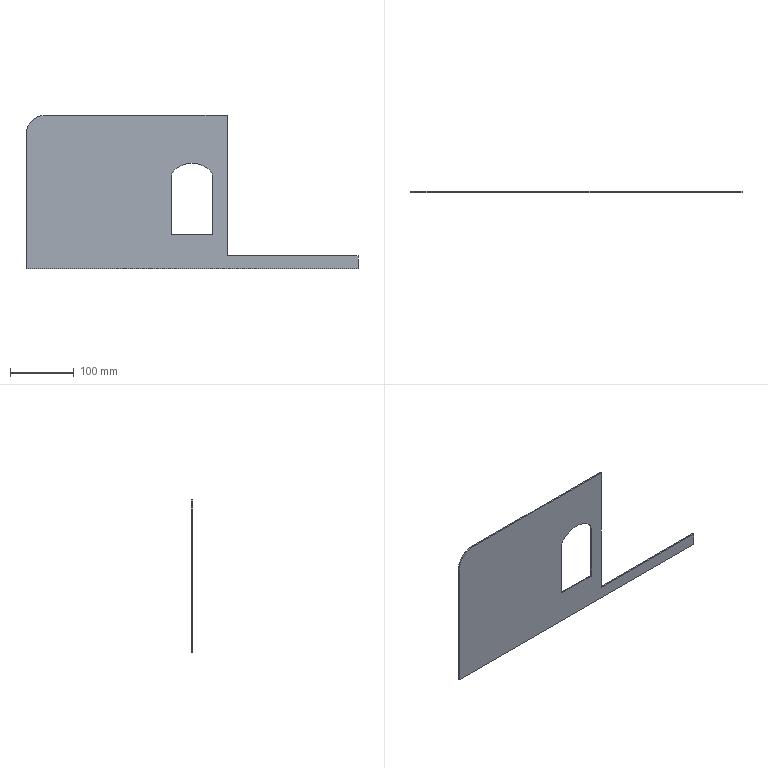Part | STEP file | A14-052 | 1 solid | 16 faces | box 520 x 2 x 240 mm | volume 145187 mm3 | plane 11 | cylinder 5 | commonest cylinder face diameters 25.5 x2 79.6 x2 60 x1
STEP:
#1=CARTESIAN_POINT('',(0.,0.,0.));
#2=DIRECTION('',(0.,0.,1.));
#3=DIRECTION('',(1.,0.,0.));
#4=AXIS2_PLACEMENT_3D('',#1,#2,#3);
#5=CARTESIAN_POINT('',(28.765,-1.,32.757));
#6=VERTEX_POINT('',#5);
#7=CARTESIAN_POINT('',(28.765,1.,32.757));
#8=VERTEX_POINT('',#7);
#9=CARTESIAN_POINT('',(28.765,-9.,32.757));
#10=DIRECTION('',(0.,1.,0.));
#11=VECTOR('',#10,1.);
#12=LINE('',#9,#11);
#13=CARTESIAN_POINT('',(0.,-9.,5.25));
#14=DIRECTION('',(0.,1.,0.));
#15=DIRECTION('',(0.,0.,1.));
#16=AXIS2_PLACEMENT_3D('',#13,#14,#15);
#17=CYLINDRICAL_SURFACE('',#16,39.8);
#18=CARTESIAN_POINT('',(0.8078,0.));
#19=DIRECTION('',(0.,1.));
#20=VECTOR('',#19,1.);
#21=LINE('',#18,#20);
#22=(GEOMETRIC_REPRESENTATION_CONTEXT(2)PARAMETRIC_REPRESENTATION_CONTEXT()REPRESENTATION_CONTEXT('',''));
#23=DEFINITIONAL_REPRESENTATION('',(#21),#22);
#24=PCURVE('',#17,#23);
#25=CARTESIAN_POINT('',(19.55,-9.,23.945));
#26=DIRECTION('',(0.,1.,0.));
#27=DIRECTION('',(0.,0.,1.));
#28=AXIS2_PLACEMENT_3D('',#25,#26,#27);
#29=CYLINDRICAL_SURFACE('',#28,12.75);
#30=CARTESIAN_POINT('',(0.8078,0.));
#31=DIRECTION('',(0.,1.));
#32=VECTOR('',#31,1.);
#33=LINE('',#30,#32);
#34=(GEOMETRIC_REPRESENTATION_CONTEXT(2)PARAMETRIC_REPRESENTATION_CONTEXT()REPRESENTATION_CONTEXT('',''));
#35=DEFINITIONAL_REPRESENTATION('',(#33),#34);
#36=PCURVE('',#29,#35);
#37=SURFACE_CURVE('',#12,(#24,#36),.PCURVE_S1.);
#38=EDGE_CURVE('',#6,#8,#37,.T.);
#39=ORIENTED_EDGE('',*,*,#38,.T.);
#40=CARTESIAN_POINT('',(0.,1.,45.05));
#41=VERTEX_POINT('',#40);
#42=CARTESIAN_POINT('',(0.,1.,5.25));
#43=DIRECTION('',(0.,1.,0.));
#44=DIRECTION('',(0.,0.,1.));
#45=AXIS2_PLACEMENT_3D('',#42,#43,#44);
#46=CIRCLE('',#45,39.8);
#47=CARTESIAN_POINT('',(0.,10.));
#48=DIRECTION('',(1.,0.));
#49=VECTOR('',#48,1.);
#50=LINE('',#47,#49);
#51=(GEOMETRIC_REPRESENTATION_CONTEXT(2)PARAMETRIC_REPRESENTATION_CONTEXT()REPRESENTATION_CONTEXT('',''));
#52=DEFINITIONAL_REPRESENTATION('',(#50),#51);
#53=PCURVE('',#17,#52);
#54=CARTESIAN_POINT('',(0.,1.,0.));
#55=DIRECTION('',(0.,1.,0.));
#56=DIRECTION('',(0.,0.,1.));
#57=AXIS2_PLACEMENT_3D('',#54,#55,#56);
#58=PLANE('',#57);
#59=CARTESIAN_POINT('',(5.25,0.));
#60=DIRECTION('',(1.,0.));
#61=AXIS2_PLACEMENT_2D('',#59,#60);
#62=CIRCLE('',#61,39.8);
#63=(GEOMETRIC_REPRESENTATION_CONTEXT(2)PARAMETRIC_REPRESENTATION_CONTEXT()REPRESENTATION_CONTEXT('',''));
#64=DEFINITIONAL_REPRESENTATION('',(#62),#63);
#65=PCURVE('',#58,#64);
#66=SURFACE_CURVE('',#46,(#53,#65),.PCURVE_S1.);
#67=EDGE_CURVE('',#41,#8,#66,.T.);
#68=ORIENTED_EDGE('',*,*,#67,.F.);
#69=CARTESIAN_POINT('',(0.,-1.,45.05));
#70=VERTEX_POINT('',#69);
#71=CARTESIAN_POINT('',(0.,-9.,45.05));
#72=DIRECTION('',(0.,1.,0.));
#73=VECTOR('',#72,1.);
#74=LINE('',#71,#73);
#75=CARTESIAN_POINT('',(0.,0.));
#76=DIRECTION('',(0.,1.));
#77=VECTOR('',#76,1.);
#78=LINE('',#75,#77);
#79=(GEOMETRIC_REPRESENTATION_CONTEXT(2)PARAMETRIC_REPRESENTATION_CONTEXT()REPRESENTATION_CONTEXT('',''));
#80=DEFINITIONAL_REPRESENTATION('',(#78),#79);
#81=PCURVE('',#17,#80);
#82=CARTESIAN_POINT('',(0.,-9.,5.25));
#83=DIRECTION('',(0.,1.,0.));
#84=DIRECTION('',(0.,0.,1.));
#85=AXIS2_PLACEMENT_3D('',#82,#83,#84);
#86=CYLINDRICAL_SURFACE('',#85,39.8);
#87=CARTESIAN_POINT('',(6.283,0.));
#88=DIRECTION('',(0.,1.));
#89=VECTOR('',#88,1.);
#90=LINE('',#87,#89);
#91=(GEOMETRIC_REPRESENTATION_CONTEXT(2)PARAMETRIC_REPRESENTATION_CONTEXT()REPRESENTATION_CONTEXT('',''));
#92=DEFINITIONAL_REPRESENTATION('',(#90),#91);
#93=PCURVE('',#86,#92);
#94=SURFACE_CURVE('',#74,(#81,#93),.PCURVE_S1.);
#95=EDGE_CURVE('',#70,#41,#94,.T.);
#96=ORIENTED_EDGE('',*,*,#95,.F.);
#97=CARTESIAN_POINT('',(0.,-1.,5.25));
#98=DIRECTION('',(0.,1.,0.));
#99=DIRECTION('',(0.,0.,1.));
#100=AXIS2_PLACEMENT_3D('',#97,#98,#99);
#101=CIRCLE('',#100,39.8);
#102=CARTESIAN_POINT('',(0.,8.));
#103=DIRECTION('',(1.,0.));
#104=VECTOR('',#103,1.);
#105=LINE('',#102,#104);
#106=(GEOMETRIC_REPRESENTATION_CONTEXT(2)PARAMETRIC_REPRESENTATION_CONTEXT()REPRESENTATION_CONTEXT('',''));
#107=DEFINITIONAL_REPRESENTATION('',(#105),#106);
#108=PCURVE('',#17,#107);
#109=CARTESIAN_POINT('',(0.,-1.,0.));
#110=DIRECTION('',(0.,1.,0.));
#111=DIRECTION('',(0.,0.,1.));
#112=AXIS2_PLACEMENT_3D('',#109,#110,#111);
#113=PLANE('',#112);
#114=CARTESIAN_POINT('',(5.25,0.));
#115=DIRECTION('',(1.,0.));
#116=AXIS2_PLACEMENT_2D('',#114,#115);
#117=CIRCLE('',#116,39.8);
#118=(GEOMETRIC_REPRESENTATION_CONTEXT(2)PARAMETRIC_REPRESENTATION_CONTEXT()REPRESENTATION_CONTEXT('',''));
#119=DEFINITIONAL_REPRESENTATION('',(#117),#118);
#120=PCURVE('',#113,#119);
#121=SURFACE_CURVE('',#101,(#108,#120),.PCURVE_S1.);
#122=EDGE_CURVE('',#70,#6,#121,.T.);
#123=ORIENTED_EDGE('',*,*,#122,.T.);
#124=EDGE_LOOP('',(#39,#68,#96,#123));
#125=FACE_BOUND('',#124,.F.);
#126=ADVANCED_FACE('',(#125),#17,.F.);
#127=CARTESIAN_POINT('',(260.,1.,-100.));
#128=VERTEX_POINT('',#127);
#129=CARTESIAN_POINT('',(260.,1.,-120.));
#130=VERTEX_POINT('',#129);
#131=CARTESIAN_POINT('',(260.,1.,-120.));
#132=DIRECTION('',(0.,0.,-1.));
#133=VECTOR('',#132,1.);
#134=LINE('',#131,#133);
#135=CARTESIAN_POINT('',(260.,1.,-120.));
#136=DIRECTION('',(-1.,0.,0.));
#137=DIRECTION('',(0.,0.,1.));
#138=AXIS2_PLACEMENT_3D('',#135,#136,#137);
#139=PLANE('',#138);
#140=CARTESIAN_POINT('',(0.,0.));
#141=DIRECTION('',(-1.,0.));
#142=VECTOR('',#141,1.);
#143=LINE('',#140,#142);
#144=(GEOMETRIC_REPRESENTATION_CONTEXT(2)PARAMETRIC_REPRESENTATION_CONTEXT()REPRESENTATION_CONTEXT('',''));
#145=DEFINITIONAL_REPRESENTATION('',(#143),#144);
#146=PCURVE('',#139,#145);
#147=CARTESIAN_POINT('',(-120.,260.));
#148=DIRECTION('',(-1.,0.));
#149=VECTOR('',#148,1.);
#150=LINE('',#147,#149);
#151=(GEOMETRIC_REPRESENTATION_CONTEXT(2)PARAMETRIC_REPRESENTATION_CONTEXT()REPRESENTATION_CONTEXT('',''));
#152=DEFINITIONAL_REPRESENTATION('',(#150),#151);
#153=PCURVE('',#58,#152);
#154=SURFACE_CURVE('',#134,(#146,#153),.PCURVE_S1.);
#155=EDGE_CURVE('',#128,#130,#154,.T.);
#156=ORIENTED_EDGE('',*,*,#155,.F.);
#157=CARTESIAN_POINT('',(260.,-1.,-100.));
#158=VERTEX_POINT('',#157);
#159=CARTESIAN_POINT('',(260.,-9.,-100.));
#160=DIRECTION('',(0.,1.,0.));
#161=VECTOR('',#160,1.);
#162=LINE('',#159,#161);
#163=CARTESIAN_POINT('',(20.,-10.));
#164=DIRECTION('',(0.,1.));
#165=VECTOR('',#164,1.);
#166=LINE('',#163,#165);
#167=(GEOMETRIC_REPRESENTATION_CONTEXT(2)PARAMETRIC_REPRESENTATION_CONTEXT()REPRESENTATION_CONTEXT('',''));
#168=DEFINITIONAL_REPRESENTATION('',(#166),#167);
#169=PCURVE('',#139,#168);
#170=CARTESIAN_POINT('',(55.,-9.,-100.));
#171=DIRECTION('',(0.,0.,-1.));
#172=DIRECTION('',(-1.,0.,0.));
#173=AXIS2_PLACEMENT_3D('',#170,#171,#172);
#174=PLANE('',#173);
#175=CARTESIAN_POINT('',(-205.,0.));
#176=DIRECTION('',(0.,1.));
#177=VECTOR('',#176,1.);
#178=LINE('',#175,#177);
#179=(GEOMETRIC_REPRESENTATION_CONTEXT(2)PARAMETRIC_REPRESENTATION_CONTEXT()REPRESENTATION_CONTEXT('',''));
#180=DEFINITIONAL_REPRESENTATION('',(#178),#179);
#181=PCURVE('',#174,#180);
#182=SURFACE_CURVE('',#162,(#169,#181),.PCURVE_S1.);
#183=EDGE_CURVE('',#158,#128,#182,.T.);
#184=ORIENTED_EDGE('',*,*,#183,.F.);
#185=CARTESIAN_POINT('',(260.,-1.,-120.));
#186=VERTEX_POINT('',#185);
#187=CARTESIAN_POINT('',(260.,-1.,-120.));
#188=DIRECTION('',(0.,0.,-1.));
#189=VECTOR('',#188,1.);
#190=LINE('',#187,#189);
#191=CARTESIAN_POINT('',(0.,-2.));
#192=DIRECTION('',(-1.,0.));
#193=VECTOR('',#192,1.);
#194=LINE('',#191,#193);
#195=(GEOMETRIC_REPRESENTATION_CONTEXT(2)PARAMETRIC_REPRESENTATION_CONTEXT()REPRESENTATION_CONTEXT('',''));
#196=DEFINITIONAL_REPRESENTATION('',(#194),#195);
#197=PCURVE('',#139,#196);
#198=CARTESIAN_POINT('',(-120.,260.));
#199=DIRECTION('',(-1.,0.));
#200=VECTOR('',#199,1.);
#201=LINE('',#198,#200);
#202=(GEOMETRIC_REPRESENTATION_CONTEXT(2)PARAMETRIC_REPRESENTATION_CONTEXT()REPRESENTATION_CONTEXT('',''));
#203=DEFINITIONAL_REPRESENTATION('',(#201),#202);
#204=PCURVE('',#113,#203);
#205=SURFACE_CURVE('',#190,(#197,#204),.PCURVE_S1.);
#206=EDGE_CURVE('',#158,#186,#205,.T.);
#207=ORIENTED_EDGE('',*,*,#206,.T.);
#208=CARTESIAN_POINT('',(260.,1.,-120.));
#209=DIRECTION('',(0.,-1.,0.));
#210=VECTOR('',#209,1.);
#211=LINE('',#208,#210);
#212=CARTESIAN_POINT('',(0.,0.));
#213=DIRECTION('',(0.,-1.));
#214=VECTOR('',#213,1.);
#215=LINE('',#212,#214);
#216=(GEOMETRIC_REPRESENTATION_CONTEXT(2)PARAMETRIC_REPRESENTATION_CONTEXT()REPRESENTATION_CONTEXT('',''));
#217=DEFINITIONAL_REPRESENTATION('',(#215),#216);
#218=PCURVE('',#139,#217);
#219=CARTESIAN_POINT('',(-260.,1.,-120.));
#220=DIRECTION('',(0.,0.,1.));
#221=DIRECTION('',(1.,0.,0.));
#222=AXIS2_PLACEMENT_3D('',#219,#220,#221);
#223=PLANE('',#222);
#224=CARTESIAN_POINT('',(520.,0.));
#225=DIRECTION('',(0.,-1.));
#226=VECTOR('',#225,1.);
#227=LINE('',#224,#226);
#228=(GEOMETRIC_REPRESENTATION_CONTEXT(2)PARAMETRIC_REPRESENTATION_CONTEXT()REPRESENTATION_CONTEXT('',''));
#229=DEFINITIONAL_REPRESENTATION('',(#227),#228);
#230=PCURVE('',#223,#229);
#231=SURFACE_CURVE('',#211,(#218,#230),.PCURVE_S1.);
#232=EDGE_CURVE('',#130,#186,#231,.T.);
#233=ORIENTED_EDGE('',*,*,#232,.F.);
#234=EDGE_LOOP('',(#156,#184,#207,#233));
#235=FACE_BOUND('',#234,.T.);
#236=ADVANCED_FACE('',(#235),#139,.F.);
#237=CARTESIAN_POINT('',(-260.,-1.,-120.));
#238=VERTEX_POINT('',#237);
#239=CARTESIAN_POINT('',(-260.,-1.,-120.));
#240=DIRECTION('',(-1.,0.,0.));
#241=VECTOR('',#240,1.);
#242=LINE('',#239,#241);
#243=CARTESIAN_POINT('',(0.,-2.));
#244=DIRECTION('',(-1.,0.));
#245=VECTOR('',#244,1.);
#246=LINE('',#243,#245);
#247=(GEOMETRIC_REPRESENTATION_CONTEXT(2)PARAMETRIC_REPRESENTATION_CONTEXT()REPRESENTATION_CONTEXT('',''));
#248=DEFINITIONAL_REPRESENTATION('',(#246),#247);
#249=PCURVE('',#223,#248);
#250=CARTESIAN_POINT('',(-120.,-260.));
#251=DIRECTION('',(0.,-1.));
#252=VECTOR('',#251,1.);
#253=LINE('',#250,#252);
#254=(GEOMETRIC_REPRESENTATION_CONTEXT(2)PARAMETRIC_REPRESENTATION_CONTEXT()REPRESENTATION_CONTEXT('',''));
#255=DEFINITIONAL_REPRESENTATION('',(#253),#254);
#256=PCURVE('',#113,#255);
#257=SURFACE_CURVE('',#242,(#249,#256),.PCURVE_S1.);
#258=EDGE_CURVE('',#186,#238,#257,.T.);
#259=ORIENTED_EDGE('',*,*,#258,.T.);
#260=CARTESIAN_POINT('',(-260.,1.,-120.));
#261=VERTEX_POINT('',#260);
#262=CARTESIAN_POINT('',(-260.,1.,-120.));
#263=DIRECTION('',(0.,-1.,0.));
#264=VECTOR('',#263,1.);
#265=LINE('',#262,#264);
#266=CARTESIAN_POINT('',(0.,0.));
#267=DIRECTION('',(0.,-1.));
#268=VECTOR('',#267,1.);
#269=LINE('',#266,#268);
#270=(GEOMETRIC_REPRESENTATION_CONTEXT(2)PARAMETRIC_REPRESENTATION_CONTEXT()REPRESENTATION_CONTEXT('',''));
#271=DEFINITIONAL_REPRESENTATION('',(#269),#270);
#272=PCURVE('',#223,#271);
#273=CARTESIAN_POINT('',(-260.,1.,-120.));
#274=DIRECTION('',(1.,0.,0.));
#275=DIRECTION('',(0.,0.,-1.));
#276=AXIS2_PLACEMENT_3D('',#273,#274,#275);
#277=PLANE('',#276);
#278=CARTESIAN_POINT('',(0.,0.));
#279=DIRECTION('',(0.,-1.));
#280=VECTOR('',#279,1.);
#281=LINE('',#278,#280);
#282=(GEOMETRIC_REPRESENTATION_CONTEXT(2)PARAMETRIC_REPRESENTATION_CONTEXT()REPRESENTATION_CONTEXT('',''));
#283=DEFINITIONAL_REPRESENTATION('',(#281),#282);
#284=PCURVE('',#277,#283);
#285=SURFACE_CURVE('',#265,(#272,#284),.PCURVE_S1.);
#286=EDGE_CURVE('',#261,#238,#285,.T.);
#287=ORIENTED_EDGE('',*,*,#286,.F.);
#288=CARTESIAN_POINT('',(-260.,1.,-120.));
#289=DIRECTION('',(-1.,0.,0.));
#290=VECTOR('',#289,1.);
#291=LINE('',#288,#290);
#292=CARTESIAN_POINT('',(0.,0.));
#293=DIRECTION('',(-1.,0.));
#294=VECTOR('',#293,1.);
#295=LINE('',#292,#294);
#296=(GEOMETRIC_REPRESENTATION_CONTEXT(2)PARAMETRIC_REPRESENTATION_CONTEXT()REPRESENTATION_CONTEXT('',''));
#297=DEFINITIONAL_REPRESENTATION('',(#295),#296);
#298=PCURVE('',#223,#297);
#299=CARTESIAN_POINT('',(-120.,-260.));
#300=DIRECTION('',(0.,-1.));
#301=VECTOR('',#300,1.);
#302=LINE('',#299,#301);
#303=(GEOMETRIC_REPRESENTATION_CONTEXT(2)PARAMETRIC_REPRESENTATION_CONTEXT()REPRESENTATION_CONTEXT('',''));
#304=DEFINITIONAL_REPRESENTATION('',(#302),#303);
#305=PCURVE('',#58,#304);
#306=SURFACE_CURVE('',#291,(#298,#305),.PCURVE_S1.);
#307=EDGE_CURVE('',#130,#261,#306,.T.);
#308=ORIENTED_EDGE('',*,*,#307,.F.);
#309=ORIENTED_EDGE('',*,*,#232,.T.);
#310=EDGE_LOOP('',(#259,#287,#308,#309));
#311=FACE_BOUND('',#310,.T.);
#312=ADVANCED_FACE('',(#311),#223,.F.);
#313=CARTESIAN_POINT('',(-260.,-1.,90.));
#314=VERTEX_POINT('',#313);
#315=CARTESIAN_POINT('',(-260.,-1.,-120.));
#316=DIRECTION('',(0.,0.,1.));
#317=VECTOR('',#316,1.);
#318=LINE('',#315,#317);
#319=CARTESIAN_POINT('',(0.,-2.));
#320=DIRECTION('',(-1.,0.));
#321=VECTOR('',#320,1.);
#322=LINE('',#319,#321);
#323=(GEOMETRIC_REPRESENTATION_CONTEXT(2)PARAMETRIC_REPRESENTATION_CONTEXT()REPRESENTATION_CONTEXT('',''));
#324=DEFINITIONAL_REPRESENTATION('',(#322),#323);
#325=PCURVE('',#277,#324);
#326=CARTESIAN_POINT('',(-120.,-260.));
#327=DIRECTION('',(1.,0.));
#328=VECTOR('',#327,1.);
#329=LINE('',#326,#328);
#330=(GEOMETRIC_REPRESENTATION_CONTEXT(2)PARAMETRIC_REPRESENTATION_CONTEXT()REPRESENTATION_CONTEXT('',''));
#331=DEFINITIONAL_REPRESENTATION('',(#329),#330);
#332=PCURVE('',#113,#331);
#333=SURFACE_CURVE('',#318,(#325,#332),.PCURVE_S1.);
#334=EDGE_CURVE('',#238,#314,#333,.T.);
#335=ORIENTED_EDGE('',*,*,#334,.T.);
#336=CARTESIAN_POINT('',(-260.,1.,90.));
#337=VERTEX_POINT('',#336);
#338=CARTESIAN_POINT('',(-260.,1.,90.));
#339=DIRECTION('',(0.,1.,0.));
#340=VECTOR('',#339,1.);
#341=LINE('',#338,#340);
#342=CARTESIAN_POINT('',(-210.,0.));
#343=DIRECTION('',(0.,1.));
#344=VECTOR('',#343,1.);
#345=LINE('',#342,#344);
#346=(GEOMETRIC_REPRESENTATION_CONTEXT(2)PARAMETRIC_REPRESENTATION_CONTEXT()REPRESENTATION_CONTEXT('',''));
#347=DEFINITIONAL_REPRESENTATION('',(#345),#346);
#348=PCURVE('',#277,#347);
#349=CARTESIAN_POINT('',(-230.,1.,90.));
#350=DIRECTION('',(0.,-1.,0.));
#351=DIRECTION('',(0.,0.,-1.));
#352=AXIS2_PLACEMENT_3D('',#349,#350,#351);
#353=CYLINDRICAL_SURFACE('',#352,30.);
#354=CARTESIAN_POINT('',(4.712,0.));
#355=DIRECTION('',(0.,-1.));
#356=VECTOR('',#355,1.);
#357=LINE('',#354,#356);
#358=(GEOMETRIC_REPRESENTATION_CONTEXT(2)PARAMETRIC_REPRESENTATION_CONTEXT()REPRESENTATION_CONTEXT('',''));
#359=DEFINITIONAL_REPRESENTATION('',(#357),#358);
#360=PCURVE('',#353,#359);
#361=SURFACE_CURVE('',#341,(#348,#360),.PCURVE_S1.);
#362=EDGE_CURVE('',#314,#337,#361,.T.);
#363=ORIENTED_EDGE('',*,*,#362,.T.);
#364=CARTESIAN_POINT('',(-260.,1.,-120.));
#365=DIRECTION('',(0.,0.,1.));
#366=VECTOR('',#365,1.);
#367=LINE('',#364,#366);
#368=CARTESIAN_POINT('',(0.,0.));
#369=DIRECTION('',(-1.,0.));
#370=VECTOR('',#369,1.);
#371=LINE('',#368,#370);
#372=(GEOMETRIC_REPRESENTATION_CONTEXT(2)PARAMETRIC_REPRESENTATION_CONTEXT()REPRESENTATION_CONTEXT('',''));
#373=DEFINITIONAL_REPRESENTATION('',(#371),#372);
#374=PCURVE('',#277,#373);
#375=CARTESIAN_POINT('',(-120.,-260.));
#376=DIRECTION('',(1.,0.));
#377=VECTOR('',#376,1.);
#378=LINE('',#375,#377);
#379=(GEOMETRIC_REPRESENTATION_CONTEXT(2)PARAMETRIC_REPRESENTATION_CONTEXT()REPRESENTATION_CONTEXT('',''));
#380=DEFINITIONAL_REPRESENTATION('',(#378),#379);
#381=PCURVE('',#58,#380);
#382=SURFACE_CURVE('',#367,(#374,#381),.PCURVE_S1.);
#383=EDGE_CURVE('',#261,#337,#382,.T.);
#384=ORIENTED_EDGE('',*,*,#383,.F.);
#385=ORIENTED_EDGE('',*,*,#286,.T.);
#386=EDGE_LOOP('',(#335,#363,#384,#385));
#387=FACE_BOUND('',#386,.T.);
#388=ADVANCED_FACE('',(#387),#277,.F.);
#389=CARTESIAN_POINT('',(-230.,-1.,120.));
#390=VERTEX_POINT('',#389);
#391=CARTESIAN_POINT('',(55.,-1.,120.));
#392=VERTEX_POINT('',#391);
#393=CARTESIAN_POINT('',(-260.,-1.,120.));
#394=DIRECTION('',(1.,0.,0.));
#395=VECTOR('',#394,1.);
#396=LINE('',#393,#395);
#397=CARTESIAN_POINT('',(-260.,1.,120.));
#398=DIRECTION('',(0.,0.,-1.));
#399=DIRECTION('',(-1.,0.,0.));
#400=AXIS2_PLACEMENT_3D('',#397,#398,#399);
#401=PLANE('',#400);
#402=CARTESIAN_POINT('',(0.,-2.));
#403=DIRECTION('',(-1.,0.));
#404=VECTOR('',#403,1.);
#405=LINE('',#402,#404);
#406=(GEOMETRIC_REPRESENTATION_CONTEXT(2)PARAMETRIC_REPRESENTATION_CONTEXT()REPRESENTATION_CONTEXT('',''));
#407=DEFINITIONAL_REPRESENTATION('',(#405),#406);
#408=PCURVE('',#401,#407);
#409=CARTESIAN_POINT('',(120.,-260.));
#410=DIRECTION('',(0.,1.));
#411=VECTOR('',#410,1.);
#412=LINE('',#409,#411);
#413=(GEOMETRIC_REPRESENTATION_CONTEXT(2)PARAMETRIC_REPRESENTATION_CONTEXT()REPRESENTATION_CONTEXT('',''));
#414=DEFINITIONAL_REPRESENTATION('',(#412),#413);
#415=PCURVE('',#113,#414);
#416=SURFACE_CURVE('',#396,(#408,#415),.PCURVE_S1.);
#417=EDGE_CURVE('',#390,#392,#416,.T.);
#418=ORIENTED_EDGE('',*,*,#417,.T.);
#419=CARTESIAN_POINT('',(55.,1.,120.));
#420=VERTEX_POINT('',#419);
#421=CARTESIAN_POINT('',(55.,-9.,120.));
#422=DIRECTION('',(0.,1.,0.));
#423=VECTOR('',#422,1.);
#424=LINE('',#421,#423);
#425=CARTESIAN_POINT('',(-315.,-10.));
#426=DIRECTION('',(0.,1.));
#427=VECTOR('',#426,1.);
#428=LINE('',#425,#427);
#429=(GEOMETRIC_REPRESENTATION_CONTEXT(2)PARAMETRIC_REPRESENTATION_CONTEXT()REPRESENTATION_CONTEXT('',''));
#430=DEFINITIONAL_REPRESENTATION('',(#428),#429);
#431=PCURVE('',#401,#430);
#432=CARTESIAN_POINT('',(55.,-9.,-100.));
#433=DIRECTION('',(-1.,0.,0.));
#434=DIRECTION('',(0.,0.,1.));
#435=AXIS2_PLACEMENT_3D('',#432,#433,#434);
#436=PLANE('',#435);
#437=CARTESIAN_POINT('',(220.,0.));
#438=DIRECTION('',(0.,1.));
#439=VECTOR('',#438,1.);
#440=LINE('',#437,#439);
#441=(GEOMETRIC_REPRESENTATION_CONTEXT(2)PARAMETRIC_REPRESENTATION_CONTEXT()REPRESENTATION_CONTEXT('',''));
#442=DEFINITIONAL_REPRESENTATION('',(#440),#441);
#443=PCURVE('',#436,#442);
#444=SURFACE_CURVE('',#424,(#431,#443),.PCURVE_S1.);
#445=EDGE_CURVE('',#392,#420,#444,.T.);
#446=ORIENTED_EDGE('',*,*,#445,.T.);
#447=CARTESIAN_POINT('',(-230.,1.,120.));
#448=VERTEX_POINT('',#447);
#449=CARTESIAN_POINT('',(-260.,1.,120.));
#450=DIRECTION('',(1.,0.,0.));
#451=VECTOR('',#450,1.);
#452=LINE('',#449,#451);
#453=CARTESIAN_POINT('',(0.,0.));
#454=DIRECTION('',(-1.,0.));
#455=VECTOR('',#454,1.);
#456=LINE('',#453,#455);
#457=(GEOMETRIC_REPRESENTATION_CONTEXT(2)PARAMETRIC_REPRESENTATION_CONTEXT()REPRESENTATION_CONTEXT('',''));
#458=DEFINITIONAL_REPRESENTATION('',(#456),#457);
#459=PCURVE('',#401,#458);
#460=CARTESIAN_POINT('',(120.,-260.));
#461=DIRECTION('',(0.,1.));
#462=VECTOR('',#461,1.);
#463=LINE('',#460,#462);
#464=(GEOMETRIC_REPRESENTATION_CONTEXT(2)PARAMETRIC_REPRESENTATION_CONTEXT()REPRESENTATION_CONTEXT('',''));
#465=DEFINITIONAL_REPRESENTATION('',(#463),#464);
#466=PCURVE('',#58,#465);
#467=SURFACE_CURVE('',#452,(#459,#466),.PCURVE_S1.);
#468=EDGE_CURVE('',#448,#420,#467,.T.);
#469=ORIENTED_EDGE('',*,*,#468,.F.);
#470=CARTESIAN_POINT('',(-230.,1.,120.));
#471=DIRECTION('',(0.,-1.,0.));
#472=VECTOR('',#471,1.);
#473=LINE('',#470,#472);
#474=CARTESIAN_POINT('',(-30.,0.));
#475=DIRECTION('',(0.,-1.));
#476=VECTOR('',#475,1.);
#477=LINE('',#474,#476);
#478=(GEOMETRIC_REPRESENTATION_CONTEXT(2)PARAMETRIC_REPRESENTATION_CONTEXT()REPRESENTATION_CONTEXT('',''));
#479=DEFINITIONAL_REPRESENTATION('',(#477),#478);
#480=PCURVE('',#401,#479);
#481=CARTESIAN_POINT('',(3.142,0.));
#482=DIRECTION('',(0.,1.));
#483=VECTOR('',#482,1.);
#484=LINE('',#481,#483);
#485=(GEOMETRIC_REPRESENTATION_CONTEXT(2)PARAMETRIC_REPRESENTATION_CONTEXT()REPRESENTATION_CONTEXT('',''));
#486=DEFINITIONAL_REPRESENTATION('',(#484),#485);
#487=PCURVE('',#353,#486);
#488=SURFACE_CURVE('',#473,(#480,#487),.PCURVE_S1.);
#489=EDGE_CURVE('',#448,#390,#488,.T.);
#490=ORIENTED_EDGE('',*,*,#489,.T.);
#491=EDGE_LOOP('',(#418,#446,#469,#490));
#492=FACE_BOUND('',#491,.T.);
#493=ADVANCED_FACE('',(#492),#401,.F.);
#494=CARTESIAN_POINT('',(55.,1.,-100.));
#495=VERTEX_POINT('',#494);
#496=CARTESIAN_POINT('',(55.,1.,-100.));
#497=DIRECTION('',(0.,0.,1.));
#498=VECTOR('',#497,1.);
#499=LINE('',#496,#498);
#500=CARTESIAN_POINT('',(-100.,55.));
#501=DIRECTION('',(1.,0.));
#502=VECTOR('',#501,1.);
#503=LINE('',#500,#502);
#504=(GEOMETRIC_REPRESENTATION_CONTEXT(2)PARAMETRIC_REPRESENTATION_CONTEXT()REPRESENTATION_CONTEXT('',''));
#505=DEFINITIONAL_REPRESENTATION('',(#503),#504);
#506=PCURVE('',#58,#505);
#507=CARTESIAN_POINT('',(0.,10.));
#508=DIRECTION('',(1.,0.));
#509=VECTOR('',#508,1.);
#510=LINE('',#507,#509);
#511=(GEOMETRIC_REPRESENTATION_CONTEXT(2)PARAMETRIC_REPRESENTATION_CONTEXT()REPRESENTATION_CONTEXT('',''));
#512=DEFINITIONAL_REPRESENTATION('',(#510),#511);
#513=PCURVE('',#436,#512);
#514=SURFACE_CURVE('',#499,(#506,#513),.PCURVE_S1.);
#515=EDGE_CURVE('',#495,#420,#514,.T.);
#516=ORIENTED_EDGE('',*,*,#515,.F.);
#517=CARTESIAN_POINT('',(55.,1.,-100.));
#518=DIRECTION('',(-1.,0.,0.));
#519=VECTOR('',#518,1.);
#520=LINE('',#517,#519);
#521=CARTESIAN_POINT('',(-100.,55.));
#522=DIRECTION('',(0.,-1.));
#523=VECTOR('',#522,1.);
#524=LINE('',#521,#523);
#525=(GEOMETRIC_REPRESENTATION_CONTEXT(2)PARAMETRIC_REPRESENTATION_CONTEXT()REPRESENTATION_CONTEXT('',''));
#526=DEFINITIONAL_REPRESENTATION('',(#524),#525);
#527=PCURVE('',#58,#526);
#528=CARTESIAN_POINT('',(0.,10.));
#529=DIRECTION('',(1.,0.));
#530=VECTOR('',#529,1.);
#531=LINE('',#528,#530);
#532=(GEOMETRIC_REPRESENTATION_CONTEXT(2)PARAMETRIC_REPRESENTATION_CONTEXT()REPRESENTATION_CONTEXT('',''));
#533=DEFINITIONAL_REPRESENTATION('',(#531),#532);
#534=PCURVE('',#174,#533);
#535=SURFACE_CURVE('',#520,(#527,#534),.PCURVE_S1.);
#536=EDGE_CURVE('',#128,#495,#535,.T.);
#537=ORIENTED_EDGE('',*,*,#536,.F.);
#538=ORIENTED_EDGE('',*,*,#155,.T.);
#539=ORIENTED_EDGE('',*,*,#307,.T.);
#540=ORIENTED_EDGE('',*,*,#383,.T.);
#541=CARTESIAN_POINT('',(-230.,1.,90.));
#542=DIRECTION('',(0.,1.,0.));
#543=DIRECTION('',(0.,0.,1.));
#544=AXIS2_PLACEMENT_3D('',#541,#542,#543);
#545=CIRCLE('',#544,30.);
#546=CARTESIAN_POINT('',(90.,-230.));
#547=DIRECTION('',(1.,0.));
#548=AXIS2_PLACEMENT_2D('',#546,#547);
#549=CIRCLE('',#548,30.);
#550=(GEOMETRIC_REPRESENTATION_CONTEXT(2)PARAMETRIC_REPRESENTATION_CONTEXT()REPRESENTATION_CONTEXT('',''));
#551=DEFINITIONAL_REPRESENTATION('',(#549),#550);
#552=PCURVE('',#58,#551);
#553=CARTESIAN_POINT('',(9.425,0.));
#554=DIRECTION('',(-1.,0.));
#555=VECTOR('',#554,1.);
#556=LINE('',#553,#555);
#557=(GEOMETRIC_REPRESENTATION_CONTEXT(2)PARAMETRIC_REPRESENTATION_CONTEXT()REPRESENTATION_CONTEXT('',''));
#558=DEFINITIONAL_REPRESENTATION('',(#556),#557);
#559=PCURVE('',#353,#558);
#560=SURFACE_CURVE('',#545,(#552,#559),.PCURVE_S1.);
#561=EDGE_CURVE('',#337,#448,#560,.T.);
#562=ORIENTED_EDGE('',*,*,#561,.T.);
#563=ORIENTED_EDGE('',*,*,#468,.T.);
#564=EDGE_LOOP('',(#516,#537,#538,#539,#540,#562,#563));
#565=FACE_BOUND('',#564,.T.);
#566=CARTESIAN_POINT('',(-32.3,1.,23.945));
#567=VERTEX_POINT('',#566);
#568=CARTESIAN_POINT('',(-28.765,1.,32.757));
#569=VERTEX_POINT('',#568);
#570=CARTESIAN_POINT('',(-19.55,1.,23.945));
#571=DIRECTION('',(0.,1.,0.));
#572=DIRECTION('',(0.,0.,1.));
#573=AXIS2_PLACEMENT_3D('',#570,#571,#572);
#574=CIRCLE('',#573,12.75);
#575=CARTESIAN_POINT('',(23.945,-19.55));
#576=DIRECTION('',(1.,0.));
#577=AXIS2_PLACEMENT_2D('',#575,#576);
#578=CIRCLE('',#577,12.75);
#579=(GEOMETRIC_REPRESENTATION_CONTEXT(2)PARAMETRIC_REPRESENTATION_CONTEXT()REPRESENTATION_CONTEXT('',''));
#580=DEFINITIONAL_REPRESENTATION('',(#578),#579);
#581=PCURVE('',#58,#580);
#582=CARTESIAN_POINT('',(-19.55,-9.,23.945));
#583=DIRECTION('',(0.,1.,0.));
#584=DIRECTION('',(0.,0.,1.));
#585=AXIS2_PLACEMENT_3D('',#582,#583,#584);
#586=CYLINDRICAL_SURFACE('',#585,12.75);
#587=CARTESIAN_POINT('',(0.,10.));
#588=DIRECTION('',(1.,0.));
#589=VECTOR('',#588,1.);
#590=LINE('',#587,#589);
#591=(GEOMETRIC_REPRESENTATION_CONTEXT(2)PARAMETRIC_REPRESENTATION_CONTEXT()REPRESENTATION_CONTEXT('',''));
#592=DEFINITIONAL_REPRESENTATION('',(#590),#591);
#593=PCURVE('',#586,#592);
#594=SURFACE_CURVE('',#574,(#581,#593),.PCURVE_S1.);
#595=EDGE_CURVE('',#567,#569,#594,.T.);
#596=ORIENTED_EDGE('',*,*,#595,.F.);
#597=CARTESIAN_POINT('',(-32.3,1.,-67.));
#598=VERTEX_POINT('',#597);
#599=CARTESIAN_POINT('',(-32.3,1.,23.945));
#600=DIRECTION('',(0.,0.,1.));
#601=VECTOR('',#600,1.);
#602=LINE('',#599,#601);
#603=CARTESIAN_POINT('',(23.945,-32.3));
#604=DIRECTION('',(1.,0.));
#605=VECTOR('',#604,1.);
#606=LINE('',#603,#605);
#607=(GEOMETRIC_REPRESENTATION_CONTEXT(2)PARAMETRIC_REPRESENTATION_CONTEXT()REPRESENTATION_CONTEXT('',''));
#608=DEFINITIONAL_REPRESENTATION('',(#606),#607);
#609=PCURVE('',#58,#608);
#610=CARTESIAN_POINT('',(-32.3,-9.,23.945));
#611=DIRECTION('',(-1.,0.,0.));
#612=DIRECTION('',(0.,0.,1.));
#613=AXIS2_PLACEMENT_3D('',#610,#611,#612);
#614=PLANE('',#613);
#615=CARTESIAN_POINT('',(0.,10.));
#616=DIRECTION('',(1.,0.));
#617=VECTOR('',#616,1.);
#618=LINE('',#615,#617);
#619=(GEOMETRIC_REPRESENTATION_CONTEXT(2)PARAMETRIC_REPRESENTATION_CONTEXT()REPRESENTATION_CONTEXT('',''));
#620=DEFINITIONAL_REPRESENTATION('',(#618),#619);
#621=PCURVE('',#614,#620);
#622=SURFACE_CURVE('',#602,(#609,#621),.PCURVE_S1.);
#623=EDGE_CURVE('',#598,#567,#622,.T.);
#624=ORIENTED_EDGE('',*,*,#623,.F.);
#625=CARTESIAN_POINT('',(32.3,1.,-67.));
#626=VERTEX_POINT('',#625);
#627=CARTESIAN_POINT('',(-32.3,1.,-67.));
#628=DIRECTION('',(-1.,0.,0.));
#629=VECTOR('',#628,1.);
#630=LINE('',#627,#629);
#631=CARTESIAN_POINT('',(-67.,-32.3));
#632=DIRECTION('',(0.,-1.));
#633=VECTOR('',#632,1.);
#634=LINE('',#631,#633);
#635=(GEOMETRIC_REPRESENTATION_CONTEXT(2)PARAMETRIC_REPRESENTATION_CONTEXT()REPRESENTATION_CONTEXT('',''));
#636=DEFINITIONAL_REPRESENTATION('',(#634),#635);
#637=PCURVE('',#58,#636);
#638=CARTESIAN_POINT('',(-32.3,-9.,-67.));
#639=DIRECTION('',(0.,0.,-1.));
#640=DIRECTION('',(-1.,0.,0.));
#641=AXIS2_PLACEMENT_3D('',#638,#639,#640);
#642=PLANE('',#641);
#643=CARTESIAN_POINT('',(0.,10.));
#644=DIRECTION('',(1.,0.));
#645=VECTOR('',#644,1.);
#646=LINE('',#643,#645);
#647=(GEOMETRIC_REPRESENTATION_CONTEXT(2)PARAMETRIC_REPRESENTATION_CONTEXT()REPRESENTATION_CONTEXT('',''));
#648=DEFINITIONAL_REPRESENTATION('',(#646),#647);
#649=PCURVE('',#642,#648);
#650=SURFACE_CURVE('',#630,(#637,#649),.PCURVE_S1.);
#651=EDGE_CURVE('',#626,#598,#650,.T.);
#652=ORIENTED_EDGE('',*,*,#651,.F.);
#653=CARTESIAN_POINT('',(32.3,1.,23.945));
#654=VERTEX_POINT('',#653);
#655=CARTESIAN_POINT('',(32.3,1.,-67.));
#656=DIRECTION('',(0.,0.,-1.));
#657=VECTOR('',#656,1.);
#658=LINE('',#655,#657);
#659=CARTESIAN_POINT('',(-67.,32.3));
#660=DIRECTION('',(-1.,0.));
#661=VECTOR('',#660,1.);
#662=LINE('',#659,#661);
#663=(GEOMETRIC_REPRESENTATION_CONTEXT(2)PARAMETRIC_REPRESENTATION_CONTEXT()REPRESENTATION_CONTEXT('',''));
#664=DEFINITIONAL_REPRESENTATION('',(#662),#663);
#665=PCURVE('',#58,#664);
#666=CARTESIAN_POINT('',(32.3,-9.,-67.));
#667=DIRECTION('',(1.,0.,0.));
#668=DIRECTION('',(0.,0.,-1.));
#669=AXIS2_PLACEMENT_3D('',#666,#667,#668);
#670=PLANE('',#669);
#671=CARTESIAN_POINT('',(0.,10.));
#672=DIRECTION('',(1.,0.));
#673=VECTOR('',#672,1.);
#674=LINE('',#671,#673);
#675=(GEOMETRIC_REPRESENTATION_CONTEXT(2)PARAMETRIC_REPRESENTATION_CONTEXT()REPRESENTATION_CONTEXT('',''));
#676=DEFINITIONAL_REPRESENTATION('',(#674),#675);
#677=PCURVE('',#670,#676);
#678=SURFACE_CURVE('',#658,(#665,#677),.PCURVE_S1.);
#679=EDGE_CURVE('',#654,#626,#678,.T.);
#680=ORIENTED_EDGE('',*,*,#679,.F.);
#681=CARTESIAN_POINT('',(19.55,1.,23.945));
#682=DIRECTION('',(0.,1.,0.));
#683=DIRECTION('',(0.,0.,1.));
#684=AXIS2_PLACEMENT_3D('',#681,#682,#683);
#685=CIRCLE('',#684,12.75);
#686=CARTESIAN_POINT('',(23.945,19.55));
#687=DIRECTION('',(1.,0.));
#688=AXIS2_PLACEMENT_2D('',#686,#687);
#689=CIRCLE('',#688,12.75);
#690=(GEOMETRIC_REPRESENTATION_CONTEXT(2)PARAMETRIC_REPRESENTATION_CONTEXT()REPRESENTATION_CONTEXT('',''));
#691=DEFINITIONAL_REPRESENTATION('',(#689),#690);
#692=PCURVE('',#58,#691);
#693=CARTESIAN_POINT('',(0.,10.));
#694=DIRECTION('',(1.,0.));
#695=VECTOR('',#694,1.);
#696=LINE('',#693,#695);
#697=(GEOMETRIC_REPRESENTATION_CONTEXT(2)PARAMETRIC_REPRESENTATION_CONTEXT()REPRESENTATION_CONTEXT('',''));
#698=DEFINITIONAL_REPRESENTATION('',(#696),#697);
#699=PCURVE('',#29,#698);
#700=SURFACE_CURVE('',#685,(#692,#699),.PCURVE_S1.);
#701=EDGE_CURVE('',#8,#654,#700,.T.);
#702=ORIENTED_EDGE('',*,*,#701,.F.);
#703=ORIENTED_EDGE('',*,*,#67,.F.);
#704=CARTESIAN_POINT('',(0.,1.,5.25));
#705=DIRECTION('',(0.,1.,0.));
#706=DIRECTION('',(0.,0.,1.));
#707=AXIS2_PLACEMENT_3D('',#704,#705,#706);
#708=CIRCLE('',#707,39.8);
#709=CARTESIAN_POINT('',(5.25,0.));
#710=DIRECTION('',(1.,0.));
#711=AXIS2_PLACEMENT_2D('',#709,#710);
#712=CIRCLE('',#711,39.8);
#713=(GEOMETRIC_REPRESENTATION_CONTEXT(2)PARAMETRIC_REPRESENTATION_CONTEXT()REPRESENTATION_CONTEXT('',''));
#714=DEFINITIONAL_REPRESENTATION('',(#712),#713);
#715=PCURVE('',#58,#714);
#716=CARTESIAN_POINT('',(0.,10.));
#717=DIRECTION('',(1.,0.));
#718=VECTOR('',#717,1.);
#719=LINE('',#716,#718);
#720=(GEOMETRIC_REPRESENTATION_CONTEXT(2)PARAMETRIC_REPRESENTATION_CONTEXT()REPRESENTATION_CONTEXT('',''));
#721=DEFINITIONAL_REPRESENTATION('',(#719),#720);
#722=PCURVE('',#86,#721);
#723=SURFACE_CURVE('',#708,(#715,#722),.PCURVE_S1.);
#724=EDGE_CURVE('',#569,#41,#723,.T.);
#725=ORIENTED_EDGE('',*,*,#724,.F.);
#726=EDGE_LOOP('',(#596,#624,#652,#680,#702,#703,#725));
#727=FACE_BOUND('',#726,.T.);
#728=ADVANCED_FACE('',(#565,#727),#58,.T.);
#729=CARTESIAN_POINT('',(-32.3,-1.,-67.));
#730=VERTEX_POINT('',#729);
#731=CARTESIAN_POINT('',(-32.3,-1.,23.945));
#732=VERTEX_POINT('',#731);
#733=CARTESIAN_POINT('',(-32.3,-1.,0.));
#734=DIRECTION('',(0.,0.,1.));
#735=VECTOR('',#734,1.);
#736=LINE('',#733,#735);
#737=CARTESIAN_POINT('',(0.,-32.3));
#738=DIRECTION('',(1.,0.));
#739=VECTOR('',#738,1.);
#740=LINE('',#737,#739);
#741=(GEOMETRIC_REPRESENTATION_CONTEXT(2)PARAMETRIC_REPRESENTATION_CONTEXT()REPRESENTATION_CONTEXT('',''));
#742=DEFINITIONAL_REPRESENTATION('',(#740),#741);
#743=PCURVE('',#113,#742);
#744=CARTESIAN_POINT('',(-23.945,8.));
#745=DIRECTION('',(1.,0.));
#746=VECTOR('',#745,1.);
#747=LINE('',#744,#746);
#748=(GEOMETRIC_REPRESENTATION_CONTEXT(2)PARAMETRIC_REPRESENTATION_CONTEXT()REPRESENTATION_CONTEXT('',''));
#749=DEFINITIONAL_REPRESENTATION('',(#747),#748);
#750=PCURVE('',#614,#749);
#751=SURFACE_CURVE('',#736,(#743,#750),.PCURVE_S1.);
#752=EDGE_CURVE('',#730,#732,#751,.T.);
#753=ORIENTED_EDGE('',*,*,#752,.T.);
#754=CARTESIAN_POINT('',(-28.765,-1.,32.757));
#755=VERTEX_POINT('',#754);
#756=CARTESIAN_POINT('',(-19.55,-1.,23.945));
#757=DIRECTION('',(0.,1.,0.));
#758=DIRECTION('',(0.,0.,1.));
#759=AXIS2_PLACEMENT_3D('',#756,#757,#758);
#760=CIRCLE('',#759,12.75);
#761=CARTESIAN_POINT('',(23.945,-19.55));
#762=DIRECTION('',(1.,0.));
#763=AXIS2_PLACEMENT_2D('',#761,#762);
#764=CIRCLE('',#763,12.75);
#765=(GEOMETRIC_REPRESENTATION_CONTEXT(2)PARAMETRIC_REPRESENTATION_CONTEXT()REPRESENTATION_CONTEXT('',''));
#766=DEFINITIONAL_REPRESENTATION('',(#764),#765);
#767=PCURVE('',#113,#766);
#768=CARTESIAN_POINT('',(0.,8.));
#769=DIRECTION('',(1.,0.));
#770=VECTOR('',#769,1.);
#771=LINE('',#768,#770);
#772=(GEOMETRIC_REPRESENTATION_CONTEXT(2)PARAMETRIC_REPRESENTATION_CONTEXT()REPRESENTATION_CONTEXT('',''));
#773=DEFINITIONAL_REPRESENTATION('',(#771),#772);
#774=PCURVE('',#586,#773);
#775=SURFACE_CURVE('',#760,(#767,#774),.PCURVE_S1.);
#776=EDGE_CURVE('',#732,#755,#775,.T.);
#777=ORIENTED_EDGE('',*,*,#776,.T.);
#778=CARTESIAN_POINT('',(0.,-1.,5.25));
#779=DIRECTION('',(0.,1.,0.));
#780=DIRECTION('',(0.,0.,1.));
#781=AXIS2_PLACEMENT_3D('',#778,#779,#780);
#782=CIRCLE('',#781,39.8);
#783=CARTESIAN_POINT('',(5.25,0.));
#784=DIRECTION('',(1.,0.));
#785=AXIS2_PLACEMENT_2D('',#783,#784);
#786=CIRCLE('',#785,39.8);
#787=(GEOMETRIC_REPRESENTATION_CONTEXT(2)PARAMETRIC_REPRESENTATION_CONTEXT()REPRESENTATION_CONTEXT('',''));
#788=DEFINITIONAL_REPRESENTATION('',(#786),#787);
#789=PCURVE('',#113,#788);
#790=CARTESIAN_POINT('',(0.,8.));
#791=DIRECTION('',(1.,0.));
#792=VECTOR('',#791,1.);
#793=LINE('',#790,#792);
#794=(GEOMETRIC_REPRESENTATION_CONTEXT(2)PARAMETRIC_REPRESENTATION_CONTEXT()REPRESENTATION_CONTEXT('',''));
#795=DEFINITIONAL_REPRESENTATION('',(#793),#794);
#796=PCURVE('',#86,#795);
#797=SURFACE_CURVE('',#782,(#789,#796),.PCURVE_S1.);
#798=EDGE_CURVE('',#755,#70,#797,.T.);
#799=ORIENTED_EDGE('',*,*,#798,.T.);
#800=ORIENTED_EDGE('',*,*,#122,.T.);
#801=CARTESIAN_POINT('',(32.3,-1.,23.945));
#802=VERTEX_POINT('',#801);
#803=CARTESIAN_POINT('',(19.55,-1.,23.945));
#804=DIRECTION('',(0.,1.,0.));
#805=DIRECTION('',(0.,0.,1.));
#806=AXIS2_PLACEMENT_3D('',#803,#804,#805);
#807=CIRCLE('',#806,12.75);
#808=CARTESIAN_POINT('',(23.945,19.55));
#809=DIRECTION('',(1.,0.));
#810=AXIS2_PLACEMENT_2D('',#808,#809);
#811=CIRCLE('',#810,12.75);
#812=(GEOMETRIC_REPRESENTATION_CONTEXT(2)PARAMETRIC_REPRESENTATION_CONTEXT()REPRESENTATION_CONTEXT('',''));
#813=DEFINITIONAL_REPRESENTATION('',(#811),#812);
#814=PCURVE('',#113,#813);
#815=CARTESIAN_POINT('',(0.,8.));
#816=DIRECTION('',(1.,0.));
#817=VECTOR('',#816,1.);
#818=LINE('',#815,#817);
#819=(GEOMETRIC_REPRESENTATION_CONTEXT(2)PARAMETRIC_REPRESENTATION_CONTEXT()REPRESENTATION_CONTEXT('',''));
#820=DEFINITIONAL_REPRESENTATION('',(#818),#819);
#821=PCURVE('',#29,#820);
#822=SURFACE_CURVE('',#807,(#814,#821),.PCURVE_S1.);
#823=EDGE_CURVE('',#6,#802,#822,.T.);
#824=ORIENTED_EDGE('',*,*,#823,.T.);
#825=CARTESIAN_POINT('',(32.3,-1.,-67.));
#826=VERTEX_POINT('',#825);
#827=CARTESIAN_POINT('',(32.3,-1.,0.));
#828=DIRECTION('',(0.,0.,-1.));
#829=VECTOR('',#828,1.);
#830=LINE('',#827,#829);
#831=CARTESIAN_POINT('',(0.,32.3));
#832=DIRECTION('',(-1.,0.));
#833=VECTOR('',#832,1.);
#834=LINE('',#831,#833);
#835=(GEOMETRIC_REPRESENTATION_CONTEXT(2)PARAMETRIC_REPRESENTATION_CONTEXT()REPRESENTATION_CONTEXT('',''));
#836=DEFINITIONAL_REPRESENTATION('',(#834),#835);
#837=PCURVE('',#113,#836);
#838=CARTESIAN_POINT('',(-67.,8.));
#839=DIRECTION('',(1.,0.));
#840=VECTOR('',#839,1.);
#841=LINE('',#838,#840);
#842=(GEOMETRIC_REPRESENTATION_CONTEXT(2)PARAMETRIC_REPRESENTATION_CONTEXT()REPRESENTATION_CONTEXT('',''));
#843=DEFINITIONAL_REPRESENTATION('',(#841),#842);
#844=PCURVE('',#670,#843);
#845=SURFACE_CURVE('',#830,(#837,#844),.PCURVE_S1.);
#846=EDGE_CURVE('',#802,#826,#845,.T.);
#847=ORIENTED_EDGE('',*,*,#846,.T.);
#848=CARTESIAN_POINT('',(0.,-1.,-67.));
#849=DIRECTION('',(-1.,0.,0.));
#850=VECTOR('',#849,1.);
#851=LINE('',#848,#850);
#852=CARTESIAN_POINT('',(-67.,0.));
#853=DIRECTION('',(0.,-1.));
#854=VECTOR('',#853,1.);
#855=LINE('',#852,#854);
#856=(GEOMETRIC_REPRESENTATION_CONTEXT(2)PARAMETRIC_REPRESENTATION_CONTEXT()REPRESENTATION_CONTEXT('',''));
#857=DEFINITIONAL_REPRESENTATION('',(#855),#856);
#858=PCURVE('',#113,#857);
#859=CARTESIAN_POINT('',(-32.3,8.));
#860=DIRECTION('',(1.,0.));
#861=VECTOR('',#860,1.);
#862=LINE('',#859,#861);
#863=(GEOMETRIC_REPRESENTATION_CONTEXT(2)PARAMETRIC_REPRESENTATION_CONTEXT()REPRESENTATION_CONTEXT('',''));
#864=DEFINITIONAL_REPRESENTATION('',(#862),#863);
#865=PCURVE('',#642,#864);
#866=SURFACE_CURVE('',#851,(#858,#865),.PCURVE_S1.);
#867=EDGE_CURVE('',#826,#730,#866,.T.);
#868=ORIENTED_EDGE('',*,*,#867,.T.);
#869=EDGE_LOOP('',(#753,#777,#799,#800,#824,#847,#868));
#870=FACE_BOUND('',#869,.T.);
#871=CARTESIAN_POINT('',(55.,-1.,-100.));
#872=VERTEX_POINT('',#871);
#873=CARTESIAN_POINT('',(0.,-1.,-100.));
#874=DIRECTION('',(-1.,0.,0.));
#875=VECTOR('',#874,1.);
#876=LINE('',#873,#875);
#877=CARTESIAN_POINT('',(-100.,0.));
#878=DIRECTION('',(0.,-1.));
#879=VECTOR('',#878,1.);
#880=LINE('',#877,#879);
#881=(GEOMETRIC_REPRESENTATION_CONTEXT(2)PARAMETRIC_REPRESENTATION_CONTEXT()REPRESENTATION_CONTEXT('',''));
#882=DEFINITIONAL_REPRESENTATION('',(#880),#881);
#883=PCURVE('',#113,#882);
#884=CARTESIAN_POINT('',(55.,8.));
#885=DIRECTION('',(1.,0.));
#886=VECTOR('',#885,1.);
#887=LINE('',#884,#886);
#888=(GEOMETRIC_REPRESENTATION_CONTEXT(2)PARAMETRIC_REPRESENTATION_CONTEXT()REPRESENTATION_CONTEXT('',''));
#889=DEFINITIONAL_REPRESENTATION('',(#887),#888);
#890=PCURVE('',#174,#889);
#891=SURFACE_CURVE('',#876,(#883,#890),.PCURVE_S1.);
#892=EDGE_CURVE('',#158,#872,#891,.T.);
#893=ORIENTED_EDGE('',*,*,#892,.T.);
#894=CARTESIAN_POINT('',(55.,-1.,0.));
#895=DIRECTION('',(0.,0.,1.));
#896=VECTOR('',#895,1.);
#897=LINE('',#894,#896);
#898=CARTESIAN_POINT('',(0.,55.));
#899=DIRECTION('',(1.,0.));
#900=VECTOR('',#899,1.);
#901=LINE('',#898,#900);
#902=(GEOMETRIC_REPRESENTATION_CONTEXT(2)PARAMETRIC_REPRESENTATION_CONTEXT()REPRESENTATION_CONTEXT('',''));
#903=DEFINITIONAL_REPRESENTATION('',(#901),#902);
#904=PCURVE('',#113,#903);
#905=CARTESIAN_POINT('',(100.,8.));
#906=DIRECTION('',(1.,0.));
#907=VECTOR('',#906,1.);
#908=LINE('',#905,#907);
#909=(GEOMETRIC_REPRESENTATION_CONTEXT(2)PARAMETRIC_REPRESENTATION_CONTEXT()REPRESENTATION_CONTEXT('',''));
#910=DEFINITIONAL_REPRESENTATION('',(#908),#909);
#911=PCURVE('',#436,#910);
#912=SURFACE_CURVE('',#897,(#904,#911),.PCURVE_S1.);
#913=EDGE_CURVE('',#872,#392,#912,.T.);
#914=ORIENTED_EDGE('',*,*,#913,.T.);
#915=ORIENTED_EDGE('',*,*,#417,.F.);
#916=CARTESIAN_POINT('',(-230.,-1.,90.));
#917=DIRECTION('',(0.,-1.,0.));
#918=DIRECTION('',(0.,0.,1.));
#919=AXIS2_PLACEMENT_3D('',#916,#917,#918);
#920=CIRCLE('',#919,30.);
#921=CARTESIAN_POINT('',(120.,-230.));
#922=CARTESIAN_POINT('',(120.,-281.962));
#923=CARTESIAN_POINT('',(75.,-255.981));
#924=CARTESIAN_POINT('',(30.,-230.));
#925=CARTESIAN_POINT('',(75.,-204.019));
#926=CARTESIAN_POINT('',(120.,-178.038));
#927=CARTESIAN_POINT('',(120.,-230.));
#928=(BOUNDED_CURVE()B_SPLINE_CURVE(2,(#921,#922,#923,#924,#925,#926,#927),.UNSPECIFIED.,.T.,.F.)B_SPLINE_CURVE_WITH_KNOTS((1,2,2,2,2,1),(-2.094,0.,2.094,4.189,6.283,8.378),.UNSPECIFIED.)CURVE()GEOMETRIC_REPRESENTATION_ITEM()RATIONAL_B_SPLINE_CURVE((1.,0.5,1.,0.5,1.,0.5,1.))REPRESENTATION_ITEM(''));
#929=(GEOMETRIC_REPRESENTATION_CONTEXT(2)PARAMETRIC_REPRESENTATION_CONTEXT()REPRESENTATION_CONTEXT('',''));
#930=DEFINITIONAL_REPRESENTATION('',(#928),#929);
#931=PCURVE('',#113,#930);
#932=CARTESIAN_POINT('',(3.142,2.));
#933=DIRECTION('',(1.,0.));
#934=VECTOR('',#933,1.);
#935=LINE('',#932,#934);
#936=(GEOMETRIC_REPRESENTATION_CONTEXT(2)PARAMETRIC_REPRESENTATION_CONTEXT()REPRESENTATION_CONTEXT('',''));
#937=DEFINITIONAL_REPRESENTATION('',(#935),#936);
#938=PCURVE('',#353,#937);
#939=SURFACE_CURVE('',#920,(#931,#938),.PCURVE_S1.);
#940=EDGE_CURVE('',#390,#314,#939,.T.);
#941=ORIENTED_EDGE('',*,*,#940,.T.);
#942=ORIENTED_EDGE('',*,*,#334,.F.);
#943=ORIENTED_EDGE('',*,*,#258,.F.);
#944=ORIENTED_EDGE('',*,*,#206,.F.);
#945=EDGE_LOOP('',(#893,#914,#915,#941,#942,#943,#944));
#946=FACE_BOUND('',#945,.T.);
#947=ADVANCED_FACE('',(#870,#946),#113,.F.);
#948=ORIENTED_EDGE('',*,*,#561,.F.);
#949=ORIENTED_EDGE('',*,*,#362,.F.);
#950=ORIENTED_EDGE('',*,*,#940,.F.);
#951=ORIENTED_EDGE('',*,*,#489,.F.);
#952=EDGE_LOOP('',(#948,#949,#950,#951));
#953=FACE_BOUND('',#952,.T.);
#954=ADVANCED_FACE('',(#953),#353,.T.);
#955=ORIENTED_EDGE('',*,*,#776,.T.);
#956=CARTESIAN_POINT('',(-28.765,-9.,32.757));
#957=DIRECTION('',(0.,1.,0.));
#958=VECTOR('',#957,1.);
#959=LINE('',#956,#958);
#960=CARTESIAN_POINT('',(5.475,0.));
#961=DIRECTION('',(0.,1.));
#962=VECTOR('',#961,1.);
#963=LINE('',#960,#962);
#964=(GEOMETRIC_REPRESENTATION_CONTEXT(2)PARAMETRIC_REPRESENTATION_CONTEXT()REPRESENTATION_CONTEXT('',''));
#965=DEFINITIONAL_REPRESENTATION('',(#963),#964);
#966=PCURVE('',#586,#965);
#967=CARTESIAN_POINT('',(5.475,0.));
#968=DIRECTION('',(0.,1.));
#969=VECTOR('',#968,1.);
#970=LINE('',#967,#969);
#971=(GEOMETRIC_REPRESENTATION_CONTEXT(2)PARAMETRIC_REPRESENTATION_CONTEXT()REPRESENTATION_CONTEXT('',''));
#972=DEFINITIONAL_REPRESENTATION('',(#970),#971);
#973=PCURVE('',#86,#972);
#974=SURFACE_CURVE('',#959,(#966,#973),.PCURVE_S1.);
#975=EDGE_CURVE('',#755,#569,#974,.T.);
#976=ORIENTED_EDGE('',*,*,#975,.T.);
#977=ORIENTED_EDGE('',*,*,#595,.F.);
#978=CARTESIAN_POINT('',(-32.3,-9.,23.945));
#979=DIRECTION('',(0.,1.,0.));
#980=VECTOR('',#979,1.);
#981=LINE('',#978,#980);
#982=CARTESIAN_POINT('',(4.712,0.));
#983=DIRECTION('',(0.,1.));
#984=VECTOR('',#983,1.);
#985=LINE('',#982,#984);
#986=(GEOMETRIC_REPRESENTATION_CONTEXT(2)PARAMETRIC_REPRESENTATION_CONTEXT()REPRESENTATION_CONTEXT('',''));
#987=DEFINITIONAL_REPRESENTATION('',(#985),#986);
#988=PCURVE('',#586,#987);
#989=CARTESIAN_POINT('',(0.,0.));
#990=DIRECTION('',(0.,1.));
#991=VECTOR('',#990,1.);
#992=LINE('',#989,#991);
#993=(GEOMETRIC_REPRESENTATION_CONTEXT(2)PARAMETRIC_REPRESENTATION_CONTEXT()REPRESENTATION_CONTEXT('',''));
#994=DEFINITIONAL_REPRESENTATION('',(#992),#993);
#995=PCURVE('',#614,#994);
#996=SURFACE_CURVE('',#981,(#988,#995),.PCURVE_S1.);
#997=EDGE_CURVE('',#732,#567,#996,.T.);
#998=ORIENTED_EDGE('',*,*,#997,.F.);
#999=EDGE_LOOP('',(#955,#976,#977,#998));
#1000=FACE_BOUND('',#999,.F.);
#1001=ADVANCED_FACE('',(#1000),#586,.F.);
#1002=CARTESIAN_POINT('',(-32.3,-9.,-67.));
#1003=DIRECTION('',(0.,1.,0.));
#1004=VECTOR('',#1003,1.);
#1005=LINE('',#1002,#1004);
#1006=CARTESIAN_POINT('',(-90.945,0.));
#1007=DIRECTION('',(0.,1.));
#1008=VECTOR('',#1007,1.);
#1009=LINE('',#1006,#1008);
#1010=(GEOMETRIC_REPRESENTATION_CONTEXT(2)PARAMETRIC_REPRESENTATION_CONTEXT()REPRESENTATION_CONTEXT('',''));
#1011=DEFINITIONAL_REPRESENTATION('',(#1009),#1010);
#1012=PCURVE('',#614,#1011);
#1013=CARTESIAN_POINT('',(0.,0.));
#1014=DIRECTION('',(0.,1.));
#1015=VECTOR('',#1014,1.);
#1016=LINE('',#1013,#1015);
#1017=(GEOMETRIC_REPRESENTATION_CONTEXT(2)PARAMETRIC_REPRESENTATION_CONTEXT()REPRESENTATION_CONTEXT('',''));
#1018=DEFINITIONAL_REPRESENTATION('',(#1016),#1017);
#1019=PCURVE('',#642,#1018);
#1020=SURFACE_CURVE('',#1005,(#1012,#1019),.PCURVE_S1.);
#1021=EDGE_CURVE('',#730,#598,#1020,.T.);
#1022=ORIENTED_EDGE('',*,*,#1021,.T.);
#1023=ORIENTED_EDGE('',*,*,#623,.T.);
#1024=ORIENTED_EDGE('',*,*,#997,.F.);
#1025=ORIENTED_EDGE('',*,*,#752,.F.);
#1026=EDGE_LOOP('',(#1022,#1023,#1024,#1025));
#1027=FACE_BOUND('',#1026,.T.);
#1028=ADVANCED_FACE('',(#1027),#614,.F.);
#1029=CARTESIAN_POINT('',(32.3,-9.,-67.));
#1030=DIRECTION('',(0.,1.,0.));
#1031=VECTOR('',#1030,1.);
#1032=LINE('',#1029,#1031);
#1033=CARTESIAN_POINT('',(-64.6,0.));
#1034=DIRECTION('',(0.,1.));
#1035=VECTOR('',#1034,1.);
#1036=LINE('',#1033,#1035);
#1037=(GEOMETRIC_REPRESENTATION_CONTEXT(2)PARAMETRIC_REPRESENTATION_CONTEXT()REPRESENTATION_CONTEXT('',''));
#1038=DEFINITIONAL_REPRESENTATION('',(#1036),#1037);
#1039=PCURVE('',#642,#1038);
#1040=CARTESIAN_POINT('',(0.,0.));
#1041=DIRECTION('',(0.,1.));
#1042=VECTOR('',#1041,1.);
#1043=LINE('',#1040,#1042);
#1044=(GEOMETRIC_REPRESENTATION_CONTEXT(2)PARAMETRIC_REPRESENTATION_CONTEXT()REPRESENTATION_CONTEXT('',''));
#1045=DEFINITIONAL_REPRESENTATION('',(#1043),#1044);
#1046=PCURVE('',#670,#1045);
#1047=SURFACE_CURVE('',#1032,(#1039,#1046),.PCURVE_S1.);
#1048=EDGE_CURVE('',#826,#626,#1047,.T.);
#1049=ORIENTED_EDGE('',*,*,#1048,.T.);
#1050=ORIENTED_EDGE('',*,*,#651,.T.);
#1051=ORIENTED_EDGE('',*,*,#1021,.F.);
#1052=ORIENTED_EDGE('',*,*,#867,.F.);
#1053=EDGE_LOOP('',(#1049,#1050,#1051,#1052));
#1054=FACE_BOUND('',#1053,.T.);
#1055=ADVANCED_FACE('',(#1054),#642,.F.);
#1056=CARTESIAN_POINT('',(32.3,-9.,23.945));
#1057=DIRECTION('',(0.,1.,0.));
#1058=VECTOR('',#1057,1.);
#1059=LINE('',#1056,#1058);
#1060=CARTESIAN_POINT('',(-90.945,0.));
#1061=DIRECTION('',(0.,1.));
#1062=VECTOR('',#1061,1.);
#1063=LINE('',#1060,#1062);
#1064=(GEOMETRIC_REPRESENTATION_CONTEXT(2)PARAMETRIC_REPRESENTATION_CONTEXT()REPRESENTATION_CONTEXT('',''));
#1065=DEFINITIONAL_REPRESENTATION('',(#1063),#1064);
#1066=PCURVE('',#670,#1065);
#1067=CARTESIAN_POINT('',(1.571,0.));
#1068=DIRECTION('',(0.,1.));
#1069=VECTOR('',#1068,1.);
#1070=LINE('',#1067,#1069);
#1071=(GEOMETRIC_REPRESENTATION_CONTEXT(2)PARAMETRIC_REPRESENTATION_CONTEXT()REPRESENTATION_CONTEXT('',''));
#1072=DEFINITIONAL_REPRESENTATION('',(#1070),#1071);
#1073=PCURVE('',#29,#1072);
#1074=SURFACE_CURVE('',#1059,(#1066,#1073),.PCURVE_S1.);
#1075=EDGE_CURVE('',#802,#654,#1074,.T.);
#1076=ORIENTED_EDGE('',*,*,#1075,.T.);
#1077=ORIENTED_EDGE('',*,*,#679,.T.);
#1078=ORIENTED_EDGE('',*,*,#1048,.F.);
#1079=ORIENTED_EDGE('',*,*,#846,.F.);
#1080=EDGE_LOOP('',(#1076,#1077,#1078,#1079));
#1081=FACE_BOUND('',#1080,.T.);
#1082=ADVANCED_FACE('',(#1081),#670,.F.);
#1083=ORIENTED_EDGE('',*,*,#823,.T.);
#1084=ORIENTED_EDGE('',*,*,#1075,.T.);
#1085=ORIENTED_EDGE('',*,*,#701,.F.);
#1086=ORIENTED_EDGE('',*,*,#38,.F.);
#1087=EDGE_LOOP('',(#1083,#1084,#1085,#1086));
#1088=FACE_BOUND('',#1087,.F.);
#1089=ADVANCED_FACE('',(#1088),#29,.F.);
#1090=ORIENTED_EDGE('',*,*,#724,.F.);
#1091=ORIENTED_EDGE('',*,*,#975,.F.);
#1092=ORIENTED_EDGE('',*,*,#798,.T.);
#1093=ORIENTED_EDGE('',*,*,#95,.T.);
#1094=EDGE_LOOP('',(#1090,#1091,#1092,#1093));
#1095=FACE_BOUND('',#1094,.F.);
#1096=ADVANCED_FACE('',(#1095),#86,.F.);
#1097=CARTESIAN_POINT('',(55.,-9.,-100.));
#1098=DIRECTION('',(0.,1.,0.));
#1099=VECTOR('',#1098,1.);
#1100=LINE('',#1097,#1099);
#1101=CARTESIAN_POINT('',(0.,0.));
#1102=DIRECTION('',(0.,1.));
#1103=VECTOR('',#1102,1.);
#1104=LINE('',#1101,#1103);
#1105=(GEOMETRIC_REPRESENTATION_CONTEXT(2)PARAMETRIC_REPRESENTATION_CONTEXT()REPRESENTATION_CONTEXT('',''));
#1106=DEFINITIONAL_REPRESENTATION('',(#1104),#1105);
#1107=PCURVE('',#436,#1106);
#1108=CARTESIAN_POINT('',(0.,0.));
#1109=DIRECTION('',(0.,1.));
#1110=VECTOR('',#1109,1.);
#1111=LINE('',#1108,#1110);
#1112=(GEOMETRIC_REPRESENTATION_CONTEXT(2)PARAMETRIC_REPRESENTATION_CONTEXT()REPRESENTATION_CONTEXT('',''));
#1113=DEFINITIONAL_REPRESENTATION('',(#1111),#1112);
#1114=PCURVE('',#174,#1113);
#1115=SURFACE_CURVE('',#1100,(#1107,#1114),.PCURVE_S1.);
#1116=EDGE_CURVE('',#872,#495,#1115,.T.);
#1117=ORIENTED_EDGE('',*,*,#1116,.T.);
#1118=ORIENTED_EDGE('',*,*,#515,.T.);
#1119=ORIENTED_EDGE('',*,*,#445,.F.);
#1120=ORIENTED_EDGE('',*,*,#913,.F.);
#1121=EDGE_LOOP('',(#1117,#1118,#1119,#1120));
#1122=FACE_BOUND('',#1121,.T.);
#1123=ADVANCED_FACE('',(#1122),#436,.F.);
#1124=ORIENTED_EDGE('',*,*,#183,.T.);
#1125=ORIENTED_EDGE('',*,*,#536,.T.);
#1126=ORIENTED_EDGE('',*,*,#1116,.F.);
#1127=ORIENTED_EDGE('',*,*,#892,.F.);
#1128=EDGE_LOOP('',(#1124,#1125,#1126,#1127));
#1129=FACE_BOUND('',#1128,.T.);
#1130=ADVANCED_FACE('',(#1129),#174,.F.);
#1131=CLOSED_SHELL('',(#126,#236,#312,#388,#493,#728,#947,#954,#1001,#1028,#1055,#1082,#1089,#1096,#1123,#1130));
#1132=MANIFOLD_SOLID_BREP('',#1131);
#1133=(LENGTH_UNIT()NAMED_UNIT(*)SI_UNIT(.MILLI.,.METRE.));
#1134=UNCERTAINTY_MEASURE_WITH_UNIT(LENGTH_MEASURE(0.0000001),#1133,'','');
#1135=(NAMED_UNIT(*)PLANE_ANGLE_UNIT()SI_UNIT($,.RADIAN.));
#1136=(NAMED_UNIT(*)SI_UNIT($,.STERADIAN.)SOLID_ANGLE_UNIT());
#1137=(GEOMETRIC_REPRESENTATION_CONTEXT(3)GLOBAL_UNCERTAINTY_ASSIGNED_CONTEXT((#1134))GLOBAL_UNIT_ASSIGNED_CONTEXT((#1133,#1135,#1136))REPRESENTATION_CONTEXT('',''));
#1138=ADVANCED_BREP_SHAPE_REPRESENTATION('',(#4,#1132),#1137);